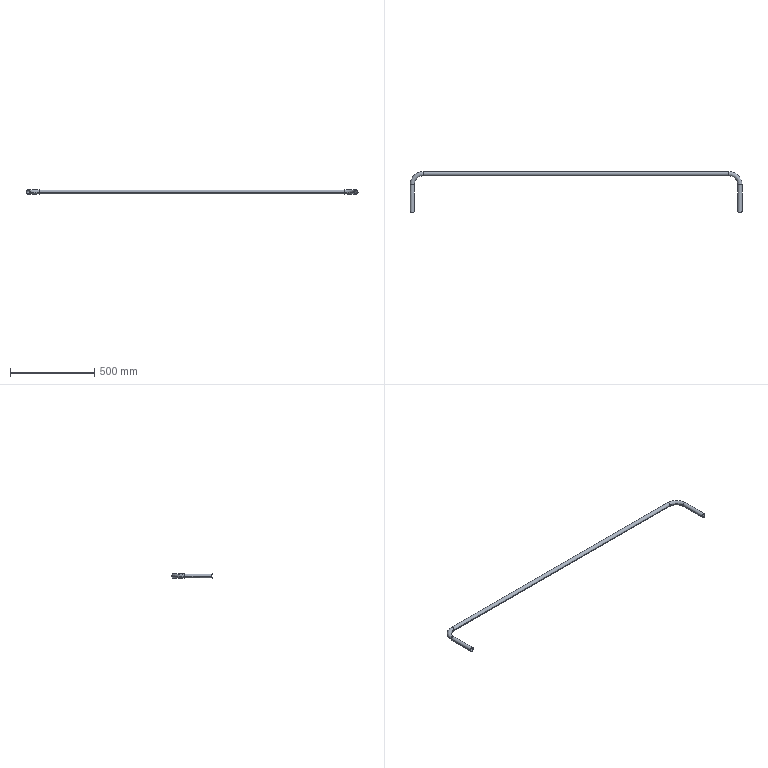Part | NX | features BREP 1 | 1 solid | 22 faces | box 1965 x 241.706 x 25.4 mm | volume 263109 mm3 | cylinder 14 | torus 8 | commonest cylinder face diameters 22.403 x6 25.4 x6 38.1 x2
STEP:
#1=CARTESIAN_POINT('',(-956.945,174.752,0.));
#2=VERTEX_POINT('',#1);
#3=CARTESIAN_POINT('',(-956.945,15.875,0.));
#4=VERTEX_POINT('',#3);
#5=CARTESIAN_POINT('',(-956.945,15.875,0.));
#6=DIRECTION('',(0.,1.,0.));
#7=VECTOR('',#6,1000.);
#8=LINE('',#5,#7);
#9=EDGE_CURVE('',#2,#4,#8,.F.);
#10=ORIENTED_EDGE('',*,*,#9,.F.);
#11=CARTESIAN_POINT('',(-982.345,174.752,0.));
#12=VERTEX_POINT('',#11);
#13=CARTESIAN_POINT('',(-969.645,174.752,0.));
#14=DIRECTION('',(0.,1.,0.));
#15=DIRECTION('',(-1.,0.,0.));
#16=AXIS2_PLACEMENT_3D('',#13,#14,#15);
#17=CIRCLE('',#16,12.7);
#18=EDGE_CURVE('',#12,#2,#17,.T.);
#19=ORIENTED_EDGE('',*,*,#18,.F.);
#20=CARTESIAN_POINT('',(-982.345,15.875,0.));
#21=VERTEX_POINT('',#20);
#22=CARTESIAN_POINT('',(-982.345,15.875,0.));
#23=DIRECTION('',(0.,1.,0.));
#24=VECTOR('',#23,1000.);
#25=LINE('',#22,#24);
#26=EDGE_CURVE('',#12,#21,#25,.F.);
#27=ORIENTED_EDGE('',*,*,#26,.T.);
#28=CARTESIAN_POINT('',(-982.345,15.875,0.));
#29=CARTESIAN_POINT('',(-982.345,15.875,0.8172));
#30=CARTESIAN_POINT('',(-982.197,15.772,2.464));
#31=CARTESIAN_POINT('',(-981.526,15.337,4.623));
#32=CARTESIAN_POINT('',(-980.908,14.947,5.892));
#33=CARTESIAN_POINT('',(-980.483,14.687,6.633));
#34=CARTESIAN_POINT('',(-980.08,14.445,7.248));
#35=CARTESIAN_POINT('',(-979.807,14.285,7.623));
#36=CARTESIAN_POINT('',(-979.423,14.062,8.115));
#37=CARTESIAN_POINT('',(-978.957,13.802,8.644));
#38=CARTESIAN_POINT('',(-978.566,13.59,9.049));
#39=CARTESIAN_POINT('',(-978.055,13.326,9.521));
#40=CARTESIAN_POINT('',(-977.617,13.108,9.893));
#41=CARTESIAN_POINT('',(-977.12,12.872,10.274));
#42=CARTESIAN_POINT('',(-976.753,12.704,10.527));
#43=CARTESIAN_POINT('',(-976.498,12.592,10.692));
#44=CARTESIAN_POINT('',(-976.434,12.564,10.734));
#45=CARTESIAN_POINT('',(-976.069,12.41,10.958));
#46=CARTESIAN_POINT('',(-975.694,12.26,11.17));
#47=CARTESIAN_POINT('',(-974.997,11.995,11.531));
#48=CARTESIAN_POINT('',(-974.162,11.714,11.889));
#49=CARTESIAN_POINT('',(-972.932,11.385,12.29));
#50=CARTESIAN_POINT('',(-971.375,11.099,12.624));
#51=CARTESIAN_POINT('',(-969.463,10.963,12.763));
#52=CARTESIAN_POINT('',(-967.657,11.135,12.582));
#53=CARTESIAN_POINT('',(-966.133,11.438,12.227));
#54=CARTESIAN_POINT('',(-964.915,11.78,11.805));
#55=CARTESIAN_POINT('',(-964.127,12.055,11.451));
#56=CARTESIAN_POINT('',(-963.454,12.315,11.092));
#57=CARTESIAN_POINT('',(-963.097,12.461,10.884));
#58=CARTESIAN_POINT('',(-962.737,12.615,10.658));
#59=CARTESIAN_POINT('',(-962.705,12.63,10.636));
#60=CARTESIAN_POINT('',(-962.476,12.732,10.485));
#61=CARTESIAN_POINT('',(-962.132,12.89,10.246));
#62=CARTESIAN_POINT('',(-961.638,13.126,9.864));
#63=CARTESIAN_POINT('',(-961.2,13.344,9.491));
#64=CARTESIAN_POINT('',(-960.795,13.554,9.112));
#65=CARTESIAN_POINT('',(-960.557,13.682,8.874));
#66=CARTESIAN_POINT('',(-960.215,13.867,8.513));
#67=CARTESIAN_POINT('',(-959.856,14.069,8.099));
#68=CARTESIAN_POINT('',(-959.472,14.291,7.608));
#69=CARTESIAN_POINT('',(-959.201,14.451,7.233));
#70=CARTESIAN_POINT('',(-958.801,14.69,6.624));
#71=CARTESIAN_POINT('',(-958.379,14.949,5.885));
#72=CARTESIAN_POINT('',(-957.946,15.222,4.997));
#73=CARTESIAN_POINT('',(-957.48,15.521,3.727));
#74=CARTESIAN_POINT('',(-957.066,15.791,2.074));
#75=CARTESIAN_POINT('',(-956.945,15.875,0.8178));
#76=CARTESIAN_POINT('',(-956.945,15.875,0.));
#77=B_SPLINE_CURVE_WITH_KNOTS('',3,(#28,#29,#30,#31,#32,#33,#34,#35,#36,#37,#38,#39,#40,#41,#42,#43,#44,#45,#46,#47,#48,#49,#50,#51,#52,#53,#54,#55,#56,#57,#58,#59,#60,#61,#62,#63,#64,#65,#66,#67,#68,#69,#70,#71,#72,#73,#74,#75,#76),.UNSPECIFIED.,.F.,.F.,(4,1,1,1,1,1,1,1,1,1,1,1,1,1,1,1,1,1,1,1,1,1,1,1,1,1,1,1,1,1,1,1,1,1,1,1,1,1,1,1,1,1,1,1,1,1,4),(0.,0.0625,0.125,0.1562,0.1719,0.1875,0.2031,0.2188,0.2344,0.25,0.2578,0.2656,0.2812,0.2969,0.3047,0.3125,0.3203,0.3281,0.3438,0.375,0.4062,0.4375,0.5,0.5625,0.5938,0.625,0.6562,0.6719,0.6797,0.6875,0.6953,0.7031,0.7188,0.7344,0.7422,0.75,0.7578,0.7656,0.7812,0.7969,0.8125,0.8281,0.8438,0.875,0.9062,0.9375,1.),.UNSPECIFIED.);
#78=EDGE_CURVE('',#21,#4,#77,.T.);
#79=ORIENTED_EDGE('',*,*,#78,.T.);
#80=EDGE_LOOP('',(#10,#19,#27,#79));
#81=FACE_BOUND('',#80,.T.);
#82=CARTESIAN_POINT('',(-969.645,0.,0.));
#83=DIRECTION('',(0.,1.,0.));
#84=DIRECTION('',(-1.,0.,0.));
#85=AXIS2_PLACEMENT_3D('',#82,#83,#84);
#86=CYLINDRICAL_SURFACE('',#85,12.7);
#87=ADVANCED_FACE('',(#81),#86,.T.);
#88=CARTESIAN_POINT('',(-982.345,15.875,0.));
#89=CARTESIAN_POINT('',(-982.345,15.875,-1.695));
#90=CARTESIAN_POINT('',(-981.677,15.422,-5.04));
#91=CARTESIAN_POINT('',(-978.692,13.557,-9.433));
#92=CARTESIAN_POINT('',(-974.201,11.514,-12.195));
#93=CARTESIAN_POINT('',(-969.57,10.77,-12.963));
#94=CARTESIAN_POINT('',(-964.988,11.553,-12.151));
#95=CARTESIAN_POINT('',(-960.544,13.589,-9.376));
#96=CARTESIAN_POINT('',(-957.6,15.431,-4.995));
#97=CARTESIAN_POINT('',(-956.945,15.875,-1.68));
#98=CARTESIAN_POINT('',(-956.945,15.875,0.));
#99=B_SPLINE_CURVE_WITH_KNOTS('',3,(#88,#89,#90,#91,#92,#93,#94,#95,#96,#97,#98),.UNSPECIFIED.,.F.,.F.,(4,1,1,1,1,1,1,1,4),(0.,0.125,0.25,0.375,0.5,0.625,0.75,0.875,1.),.UNSPECIFIED.);
#100=EDGE_CURVE('',#4,#21,#99,.F.);
#101=ORIENTED_EDGE('',*,*,#100,.F.);
#102=ORIENTED_EDGE('',*,*,#78,.F.);
#103=EDGE_LOOP('',(#101,#102));
#104=FACE_BOUND('',#103,.T.);
#105=CARTESIAN_POINT('',(-958.444,15.875,0.));
#106=VERTEX_POINT('',#105);
#107=CARTESIAN_POINT('',(-980.846,15.875,0.));
#108=VERTEX_POINT('',#107);
#109=CARTESIAN_POINT('',(-980.846,15.875,0.));
#110=CARTESIAN_POINT('',(-980.846,15.875,1.513));
#111=CARTESIAN_POINT('',(-980.232,15.505,4.51));
#112=CARTESIAN_POINT('',(-977.61,14.087,8.313));
#113=CARTESIAN_POINT('',(-973.75,12.609,10.717));
#114=CARTESIAN_POINT('',(-969.642,12.045,11.446));
#115=CARTESIAN_POINT('',(-965.514,12.615,10.707));
#116=CARTESIAN_POINT('',(-961.681,14.087,8.312));
#117=CARTESIAN_POINT('',(-959.051,15.509,4.496));
#118=CARTESIAN_POINT('',(-958.444,15.875,1.51));
#119=CARTESIAN_POINT('',(-958.444,15.875,0.));
#120=B_SPLINE_CURVE_WITH_KNOTS('',3,(#109,#110,#111,#112,#113,#114,#115,#116,#117,#118,#119),.UNSPECIFIED.,.F.,.F.,(4,1,1,1,1,1,1,1,4),(0.,0.125,0.25,0.375,0.5,0.625,0.75,0.875,1.),.UNSPECIFIED.);
#121=EDGE_CURVE('',#106,#108,#120,.F.);
#122=ORIENTED_EDGE('',*,*,#121,.F.);
#123=CARTESIAN_POINT('',(-958.444,15.875,0.));
#124=CARTESIAN_POINT('',(-958.444,15.875,-1.476));
#125=CARTESIAN_POINT('',(-959.015,15.532,-4.378));
#126=CARTESIAN_POINT('',(-961.576,14.135,-8.222));
#127=CARTESIAN_POINT('',(-965.462,12.632,-10.686));
#128=CARTESIAN_POINT('',(-969.537,12.04,-11.451));
#129=CARTESIAN_POINT('',(-973.803,12.611,-10.719));
#130=CARTESIAN_POINT('',(-977.735,14.147,-8.202));
#131=CARTESIAN_POINT('',(-980.277,15.533,-4.367));
#132=CARTESIAN_POINT('',(-980.846,15.875,-1.472));
#133=CARTESIAN_POINT('',(-980.846,15.875,0.));
#134=B_SPLINE_CURVE_WITH_KNOTS('',3,(#123,#124,#125,#126,#127,#128,#129,#130,#131,#132,#133),.UNSPECIFIED.,.F.,.F.,(4,1,1,1,1,1,1,1,4),(0.,0.125,0.25,0.375,0.5,0.625,0.75,0.875,1.),.UNSPECIFIED.);
#135=EDGE_CURVE('',#108,#106,#134,.F.);
#136=ORIENTED_EDGE('',*,*,#135,.F.);
#137=EDGE_LOOP('',(#122,#136));
#138=FACE_BOUND('',#137,.T.);
#139=CARTESIAN_POINT('',(1178.814,-3.175,0.));
#140=DIRECTION('',(1.,0.,0.));
#141=DIRECTION('',(0.,0.,-1.));
#142=AXIS2_PLACEMENT_3D('',#139,#140,#141);
#143=CYLINDRICAL_SURFACE('',#142,19.05);
#144=ADVANCED_FACE('',(#104,#138),#143,.F.);
#145=CARTESIAN_POINT('',(982.345,15.875,0.));
#146=VERTEX_POINT('',#145);
#147=CARTESIAN_POINT('',(956.945,15.875,0.));
#148=VERTEX_POINT('',#147);
#149=CARTESIAN_POINT('',(956.945,15.875,0.));
#150=CARTESIAN_POINT('',(956.945,15.875,-1.694));
#151=CARTESIAN_POINT('',(957.616,15.42,-5.043));
#152=CARTESIAN_POINT('',(960.585,13.565,-9.414));
#153=CARTESIAN_POINT('',(965.036,11.537,-12.168));
#154=CARTESIAN_POINT('',(969.617,10.769,-12.963));
#155=CARTESIAN_POINT('',(974.249,11.53,-12.178));
#156=CARTESIAN_POINT('',(978.733,13.581,-9.394));
#157=CARTESIAN_POINT('',(981.691,15.432,-4.995));
#158=CARTESIAN_POINT('',(982.345,15.875,-1.682));
#159=CARTESIAN_POINT('',(982.345,15.875,0.));
#160=B_SPLINE_CURVE_WITH_KNOTS('',3,(#149,#150,#151,#152,#153,#154,#155,#156,#157,#158,#159),.UNSPECIFIED.,.F.,.F.,(4,1,1,1,1,1,1,1,4),(0.,0.125,0.25,0.375,0.5,0.625,0.75,0.875,1.),.UNSPECIFIED.);
#161=EDGE_CURVE('',#146,#148,#160,.F.);
#162=ORIENTED_EDGE('',*,*,#161,.F.);
#163=CARTESIAN_POINT('',(982.345,15.875,0.));
#164=CARTESIAN_POINT('',(982.345,15.875,1.704));
#165=CARTESIAN_POINT('',(981.657,15.408,5.088));
#166=CARTESIAN_POINT('',(978.7,13.566,9.4));
#167=CARTESIAN_POINT('',(974.367,11.587,12.109));
#168=CARTESIAN_POINT('',(969.865,10.768,12.966));
#169=CARTESIAN_POINT('',(965.12,11.494,12.222));
#170=CARTESIAN_POINT('',(960.591,13.562,9.425));
#171=CARTESIAN_POINT('',(957.623,15.415,5.06));
#172=CARTESIAN_POINT('',(956.945,15.875,1.699));
#173=CARTESIAN_POINT('',(956.945,15.875,0.));
#174=B_SPLINE_CURVE_WITH_KNOTS('',3,(#163,#164,#165,#166,#167,#168,#169,#170,#171,#172,#173),.UNSPECIFIED.,.F.,.F.,(4,1,1,1,1,1,1,1,4),(0.,0.125,0.25,0.375,0.5,0.625,0.75,0.875,1.),.UNSPECIFIED.);
#175=EDGE_CURVE('',#148,#146,#174,.F.);
#176=ORIENTED_EDGE('',*,*,#175,.F.);
#177=EDGE_LOOP('',(#162,#176));
#178=FACE_BOUND('',#177,.T.);
#179=CARTESIAN_POINT('',(980.846,15.875,0.));
#180=VERTEX_POINT('',#179);
#181=CARTESIAN_POINT('',(958.444,15.875,0.));
#182=VERTEX_POINT('',#181);
#183=CARTESIAN_POINT('',(958.444,15.875,0.));
#184=CARTESIAN_POINT('',(958.444,15.875,1.51));
#185=CARTESIAN_POINT('',(959.051,15.509,4.496));
#186=CARTESIAN_POINT('',(961.681,14.087,8.312));
#187=CARTESIAN_POINT('',(965.514,12.615,10.707));
#188=CARTESIAN_POINT('',(969.642,12.045,11.446));
#189=CARTESIAN_POINT('',(973.75,12.609,10.717));
#190=CARTESIAN_POINT('',(977.61,14.087,8.313));
#191=CARTESIAN_POINT('',(980.232,15.505,4.51));
#192=CARTESIAN_POINT('',(980.846,15.875,1.514));
#193=CARTESIAN_POINT('',(980.846,15.875,0.));
#194=B_SPLINE_CURVE_WITH_KNOTS('',3,(#183,#184,#185,#186,#187,#188,#189,#190,#191,#192,#193),.UNSPECIFIED.,.F.,.F.,(4,1,1,1,1,1,1,1,4),(0.,0.125,0.25,0.375,0.5,0.625,0.75,0.875,1.),.UNSPECIFIED.);
#195=EDGE_CURVE('',#180,#182,#194,.F.);
#196=ORIENTED_EDGE('',*,*,#195,.F.);
#197=CARTESIAN_POINT('',(980.846,15.875,0.));
#198=CARTESIAN_POINT('',(980.846,15.875,-1.475));
#199=CARTESIAN_POINT('',(980.274,15.532,-4.378));
#200=CARTESIAN_POINT('',(977.72,14.139,-8.214));
#201=CARTESIAN_POINT('',(973.844,12.635,-10.682));
#202=CARTESIAN_POINT('',(969.746,12.04,-11.45));
#203=CARTESIAN_POINT('',(965.517,12.604,-10.728));
#204=CARTESIAN_POINT('',(961.566,14.14,-8.217));
#205=CARTESIAN_POINT('',(959.016,15.531,-4.376));
#206=CARTESIAN_POINT('',(958.444,15.875,-1.476));
#207=CARTESIAN_POINT('',(958.444,15.875,0.));
#208=B_SPLINE_CURVE_WITH_KNOTS('',3,(#197,#198,#199,#200,#201,#202,#203,#204,#205,#206,#207),.UNSPECIFIED.,.F.,.F.,(4,1,1,1,1,1,1,1,4),(0.,0.125,0.25,0.375,0.5,0.625,0.75,0.875,1.),.UNSPECIFIED.);
#209=EDGE_CURVE('',#182,#180,#208,.F.);
#210=ORIENTED_EDGE('',*,*,#209,.F.);
#211=EDGE_LOOP('',(#196,#210));
#212=FACE_BOUND('',#211,.T.);
#213=CARTESIAN_POINT('',(1178.814,-3.175,0.));
#214=DIRECTION('',(1.,0.,0.));
#215=DIRECTION('',(0.,0.,-1.));
#216=AXIS2_PLACEMENT_3D('',#213,#214,#215);
#217=CYLINDRICAL_SURFACE('',#216,19.05);
#218=ADVANCED_FACE('',(#178,#212),#217,.F.);
#219=ORIENTED_EDGE('',*,*,#26,.F.);
#220=CARTESIAN_POINT('',(-969.645,174.752,0.));
#221=DIRECTION('',(0.,1.,0.));
#222=DIRECTION('',(1.,0.,0.));
#223=AXIS2_PLACEMENT_3D('',#220,#221,#222);
#224=CIRCLE('',#223,12.7);
#225=EDGE_CURVE('',#2,#12,#224,.T.);
#226=ORIENTED_EDGE('',*,*,#225,.F.);
#227=ORIENTED_EDGE('',*,*,#9,.T.);
#228=ORIENTED_EDGE('',*,*,#100,.T.);
#229=EDGE_LOOP('',(#219,#226,#227,#228));
#230=FACE_BOUND('',#229,.T.);
#231=CARTESIAN_POINT('',(-969.645,0.,0.));
#232=DIRECTION('',(0.,1.,0.));
#233=DIRECTION('',(-1.,0.,0.));
#234=AXIS2_PLACEMENT_3D('',#231,#232,#233);
#235=CYLINDRICAL_SURFACE('',#234,12.7);
#236=ADVANCED_FACE('',(#230),#235,.T.);
#237=CARTESIAN_POINT('',(-904.367,252.73,0.));
#238=VERTEX_POINT('',#237);
#239=CARTESIAN_POINT('',(-904.367,174.752,0.));
#240=DIRECTION('',(0.,0.,-1.));
#241=DIRECTION('',(-1.,0.,0.));
#242=AXIS2_PLACEMENT_3D('',#239,#240,#241);
#243=CIRCLE('',#242,77.978);
#244=EDGE_CURVE('',#12,#238,#243,.T.);
#245=ORIENTED_EDGE('',*,*,#244,.T.);
#246=CARTESIAN_POINT('',(-904.367,227.33,0.));
#247=VERTEX_POINT('',#246);
#248=CARTESIAN_POINT('',(-904.367,240.03,0.));
#249=DIRECTION('',(1.,0.,0.));
#250=DIRECTION('',(0.,-1.,0.));
#251=AXIS2_PLACEMENT_3D('',#248,#249,#250);
#252=CIRCLE('',#251,12.7);
#253=EDGE_CURVE('',#247,#238,#252,.T.);
#254=ORIENTED_EDGE('',*,*,#253,.F.);
#255=CARTESIAN_POINT('',(-904.367,174.752,0.));
#256=DIRECTION('',(0.,0.,-1.));
#257=DIRECTION('',(-1.,0.,0.));
#258=AXIS2_PLACEMENT_3D('',#255,#256,#257);
#259=CIRCLE('',#258,52.578);
#260=EDGE_CURVE('',#2,#247,#259,.T.);
#261=ORIENTED_EDGE('',*,*,#260,.F.);
#262=ORIENTED_EDGE('',*,*,#225,.T.);
#263=EDGE_LOOP('',(#245,#254,#261,#262));
#264=FACE_BOUND('',#263,.T.);
#265=CARTESIAN_POINT('',(-904.367,174.752,0.));
#266=DIRECTION('',(0.,0.,-1.));
#267=DIRECTION('',(1.,0.,0.));
#268=AXIS2_PLACEMENT_3D('',#265,#266,#267);
#269=TOROIDAL_SURFACE('',#268,65.278,12.7);
#270=ADVANCED_FACE('',(#264),#269,.T.);
#271=ORIENTED_EDGE('',*,*,#260,.T.);
#272=CARTESIAN_POINT('',(-904.367,240.03,0.));
#273=DIRECTION('',(1.,0.,0.));
#274=DIRECTION('',(0.,1.,0.));
#275=AXIS2_PLACEMENT_3D('',#272,#273,#274);
#276=CIRCLE('',#275,12.7);
#277=EDGE_CURVE('',#238,#247,#276,.T.);
#278=ORIENTED_EDGE('',*,*,#277,.F.);
#279=ORIENTED_EDGE('',*,*,#244,.F.);
#280=ORIENTED_EDGE('',*,*,#18,.T.);
#281=EDGE_LOOP('',(#271,#278,#279,#280));
#282=FACE_BOUND('',#281,.T.);
#283=CARTESIAN_POINT('',(-904.367,174.752,0.));
#284=DIRECTION('',(0.,0.,-1.));
#285=DIRECTION('',(1.,0.,0.));
#286=AXIS2_PLACEMENT_3D('',#283,#284,#285);
#287=TOROIDAL_SURFACE('',#286,65.278,12.7);
#288=ADVANCED_FACE('',(#282),#287,.T.);
#289=CARTESIAN_POINT('',(904.367,227.33,0.));
#290=VERTEX_POINT('',#289);
#291=CARTESIAN_POINT('',(-904.367,227.33,0.));
#292=DIRECTION('',(1.,0.,0.));
#293=VECTOR('',#292,1000.);
#294=LINE('',#291,#293);
#295=EDGE_CURVE('',#247,#290,#294,.T.);
#296=ORIENTED_EDGE('',*,*,#295,.T.);
#297=CARTESIAN_POINT('',(904.367,252.73,0.));
#298=VERTEX_POINT('',#297);
#299=CARTESIAN_POINT('',(904.367,240.03,0.));
#300=DIRECTION('',(1.,0.,0.));
#301=DIRECTION('',(0.,1.,0.));
#302=AXIS2_PLACEMENT_3D('',#299,#300,#301);
#303=CIRCLE('',#302,12.7);
#304=EDGE_CURVE('',#298,#290,#303,.T.);
#305=ORIENTED_EDGE('',*,*,#304,.F.);
#306=CARTESIAN_POINT('',(-904.367,252.73,0.));
#307=DIRECTION('',(1.,0.,0.));
#308=VECTOR('',#307,1000.);
#309=LINE('',#306,#308);
#310=EDGE_CURVE('',#238,#298,#309,.T.);
#311=ORIENTED_EDGE('',*,*,#310,.F.);
#312=ORIENTED_EDGE('',*,*,#277,.T.);
#313=EDGE_LOOP('',(#296,#305,#311,#312));
#314=FACE_BOUND('',#313,.T.);
#315=CARTESIAN_POINT('',(-904.367,240.03,0.));
#316=DIRECTION('',(1.,0.,0.));
#317=DIRECTION('',(0.,1.,0.));
#318=AXIS2_PLACEMENT_3D('',#315,#316,#317);
#319=CYLINDRICAL_SURFACE('',#318,12.7);
#320=ADVANCED_FACE('',(#314),#319,.T.);
#321=ORIENTED_EDGE('',*,*,#310,.T.);
#322=CARTESIAN_POINT('',(904.367,240.03,0.));
#323=DIRECTION('',(1.,0.,0.));
#324=DIRECTION('',(0.,-1.,0.));
#325=AXIS2_PLACEMENT_3D('',#322,#323,#324);
#326=CIRCLE('',#325,12.7);
#327=EDGE_CURVE('',#290,#298,#326,.T.);
#328=ORIENTED_EDGE('',*,*,#327,.F.);
#329=ORIENTED_EDGE('',*,*,#295,.F.);
#330=ORIENTED_EDGE('',*,*,#253,.T.);
#331=EDGE_LOOP('',(#321,#328,#329,#330));
#332=FACE_BOUND('',#331,.T.);
#333=CARTESIAN_POINT('',(-904.367,240.03,0.));
#334=DIRECTION('',(1.,0.,0.));
#335=DIRECTION('',(0.,1.,0.));
#336=AXIS2_PLACEMENT_3D('',#333,#334,#335);
#337=CYLINDRICAL_SURFACE('',#336,12.7);
#338=ADVANCED_FACE('',(#332),#337,.T.);
#339=CARTESIAN_POINT('',(982.345,174.752,0.));
#340=VERTEX_POINT('',#339);
#341=CARTESIAN_POINT('',(904.367,174.752,0.));
#342=DIRECTION('',(0.,0.,-1.));
#343=DIRECTION('',(0.,1.,0.));
#344=AXIS2_PLACEMENT_3D('',#341,#342,#343);
#345=CIRCLE('',#344,77.978);
#346=EDGE_CURVE('',#340,#298,#345,.F.);
#347=ORIENTED_EDGE('',*,*,#346,.F.);
#348=CARTESIAN_POINT('',(956.945,174.752,0.));
#349=VERTEX_POINT('',#348);
#350=CARTESIAN_POINT('',(969.645,174.752,0.));
#351=DIRECTION('',(0.,-1.,0.));
#352=DIRECTION('',(-1.,0.,0.));
#353=AXIS2_PLACEMENT_3D('',#350,#351,#352);
#354=CIRCLE('',#353,12.7);
#355=EDGE_CURVE('',#349,#340,#354,.T.);
#356=ORIENTED_EDGE('',*,*,#355,.F.);
#357=CARTESIAN_POINT('',(904.367,174.752,0.));
#358=DIRECTION('',(0.,0.,-1.));
#359=DIRECTION('',(0.,1.,0.));
#360=AXIS2_PLACEMENT_3D('',#357,#358,#359);
#361=CIRCLE('',#360,52.578);
#362=EDGE_CURVE('',#349,#290,#361,.F.);
#363=ORIENTED_EDGE('',*,*,#362,.T.);
#364=ORIENTED_EDGE('',*,*,#327,.T.);
#365=EDGE_LOOP('',(#347,#356,#363,#364));
#366=FACE_BOUND('',#365,.T.);
#367=CARTESIAN_POINT('',(904.367,174.752,0.));
#368=DIRECTION('',(0.,0.,-1.));
#369=DIRECTION('',(0.,-1.,0.));
#370=AXIS2_PLACEMENT_3D('',#367,#368,#369);
#371=TOROIDAL_SURFACE('',#370,65.278,12.7);
#372=ADVANCED_FACE('',(#366),#371,.T.);
#373=ORIENTED_EDGE('',*,*,#362,.F.);
#374=CARTESIAN_POINT('',(969.645,174.752,0.));
#375=DIRECTION('',(0.,-1.,0.));
#376=DIRECTION('',(1.,0.,0.));
#377=AXIS2_PLACEMENT_3D('',#374,#375,#376);
#378=CIRCLE('',#377,12.7);
#379=EDGE_CURVE('',#340,#349,#378,.T.);
#380=ORIENTED_EDGE('',*,*,#379,.F.);
#381=ORIENTED_EDGE('',*,*,#346,.T.);
#382=ORIENTED_EDGE('',*,*,#304,.T.);
#383=EDGE_LOOP('',(#373,#380,#381,#382));
#384=FACE_BOUND('',#383,.T.);
#385=CARTESIAN_POINT('',(904.367,174.752,0.));
#386=DIRECTION('',(0.,0.,-1.));
#387=DIRECTION('',(0.,-1.,0.));
#388=AXIS2_PLACEMENT_3D('',#385,#386,#387);
#389=TOROIDAL_SURFACE('',#388,65.278,12.7);
#390=ADVANCED_FACE('',(#384),#389,.T.);
#391=CARTESIAN_POINT('',(982.345,174.752,0.));
#392=DIRECTION('',(0.,-1.,0.));
#393=VECTOR('',#392,1000.);
#394=LINE('',#391,#393);
#395=EDGE_CURVE('',#146,#340,#394,.F.);
#396=ORIENTED_EDGE('',*,*,#395,.T.);
#397=ORIENTED_EDGE('',*,*,#379,.T.);
#398=CARTESIAN_POINT('',(956.945,174.752,0.));
#399=DIRECTION('',(0.,-1.,0.));
#400=VECTOR('',#399,1000.);
#401=LINE('',#398,#400);
#402=EDGE_CURVE('',#148,#349,#401,.F.);
#403=ORIENTED_EDGE('',*,*,#402,.F.);
#404=ORIENTED_EDGE('',*,*,#175,.T.);
#405=EDGE_LOOP('',(#396,#397,#403,#404));
#406=FACE_BOUND('',#405,.T.);
#407=CARTESIAN_POINT('',(969.645,174.752,0.));
#408=DIRECTION('',(0.,-1.,0.));
#409=DIRECTION('',(1.,0.,0.));
#410=AXIS2_PLACEMENT_3D('',#407,#408,#409);
#411=CYLINDRICAL_SURFACE('',#410,12.7);
#412=ADVANCED_FACE('',(#406),#411,.T.);
#413=ORIENTED_EDGE('',*,*,#402,.T.);
#414=ORIENTED_EDGE('',*,*,#355,.T.);
#415=ORIENTED_EDGE('',*,*,#395,.F.);
#416=ORIENTED_EDGE('',*,*,#161,.T.);
#417=EDGE_LOOP('',(#413,#414,#415,#416));
#418=FACE_BOUND('',#417,.T.);
#419=CARTESIAN_POINT('',(969.645,174.752,0.));
#420=DIRECTION('',(0.,-1.,0.));
#421=DIRECTION('',(1.,0.,0.));
#422=AXIS2_PLACEMENT_3D('',#419,#420,#421);
#423=CYLINDRICAL_SURFACE('',#422,12.7);
#424=ADVANCED_FACE('',(#418),#423,.T.);
#425=CARTESIAN_POINT('',(-958.444,174.752,0.));
#426=VERTEX_POINT('',#425);
#427=CARTESIAN_POINT('',(-958.444,15.875,0.));
#428=DIRECTION('',(0.,1.,0.));
#429=VECTOR('',#428,1000.);
#430=LINE('',#427,#429);
#431=EDGE_CURVE('',#426,#106,#430,.F.);
#432=ORIENTED_EDGE('',*,*,#431,.F.);
#433=CARTESIAN_POINT('',(-980.846,174.752,0.));
#434=VERTEX_POINT('',#433);
#435=CARTESIAN_POINT('',(-969.645,174.752,0.));
#436=DIRECTION('',(0.,-1.,0.));
#437=DIRECTION('',(-1.,0.,0.));
#438=AXIS2_PLACEMENT_3D('',#435,#436,#437);
#439=CIRCLE('',#438,11.201);
#440=EDGE_CURVE('',#434,#426,#439,.T.);
#441=ORIENTED_EDGE('',*,*,#440,.F.);
#442=CARTESIAN_POINT('',(-980.846,15.875,0.));
#443=DIRECTION('',(0.,1.,0.));
#444=VECTOR('',#443,1000.);
#445=LINE('',#442,#444);
#446=EDGE_CURVE('',#434,#108,#445,.F.);
#447=ORIENTED_EDGE('',*,*,#446,.T.);
#448=ORIENTED_EDGE('',*,*,#135,.T.);
#449=EDGE_LOOP('',(#432,#441,#447,#448));
#450=FACE_BOUND('',#449,.T.);
#451=CARTESIAN_POINT('',(-969.645,0.,0.));
#452=DIRECTION('',(0.,1.,0.));
#453=DIRECTION('',(-1.,0.,0.));
#454=AXIS2_PLACEMENT_3D('',#451,#452,#453);
#455=CYLINDRICAL_SURFACE('',#454,11.201);
#456=ADVANCED_FACE('',(#450),#455,.F.);
#457=ORIENTED_EDGE('',*,*,#446,.F.);
#458=CARTESIAN_POINT('',(-969.645,174.752,0.));
#459=DIRECTION('',(0.,-1.,0.));
#460=DIRECTION('',(1.,0.,0.));
#461=AXIS2_PLACEMENT_3D('',#458,#459,#460);
#462=CIRCLE('',#461,11.201);
#463=EDGE_CURVE('',#426,#434,#462,.T.);
#464=ORIENTED_EDGE('',*,*,#463,.F.);
#465=ORIENTED_EDGE('',*,*,#431,.T.);
#466=ORIENTED_EDGE('',*,*,#121,.T.);
#467=EDGE_LOOP('',(#457,#464,#465,#466));
#468=FACE_BOUND('',#467,.T.);
#469=CARTESIAN_POINT('',(-969.645,0.,0.));
#470=DIRECTION('',(0.,1.,0.));
#471=DIRECTION('',(-1.,0.,0.));
#472=AXIS2_PLACEMENT_3D('',#469,#470,#471);
#473=CYLINDRICAL_SURFACE('',#472,11.201);
#474=ADVANCED_FACE('',(#468),#473,.F.);
#475=CARTESIAN_POINT('',(-904.367,251.231,0.));
#476=VERTEX_POINT('',#475);
#477=CARTESIAN_POINT('',(-904.367,174.752,0.));
#478=DIRECTION('',(0.,0.,-1.));
#479=DIRECTION('',(-1.,0.,0.));
#480=AXIS2_PLACEMENT_3D('',#477,#478,#479);
#481=CIRCLE('',#480,76.479);
#482=EDGE_CURVE('',#434,#476,#481,.T.);
#483=ORIENTED_EDGE('',*,*,#482,.T.);
#484=CARTESIAN_POINT('',(-904.367,228.829,0.));
#485=VERTEX_POINT('',#484);
#486=CARTESIAN_POINT('',(-904.367,240.03,0.));
#487=DIRECTION('',(-1.,0.,0.));
#488=DIRECTION('',(0.,-1.,0.));
#489=AXIS2_PLACEMENT_3D('',#486,#487,#488);
#490=CIRCLE('',#489,11.201);
#491=EDGE_CURVE('',#485,#476,#490,.T.);
#492=ORIENTED_EDGE('',*,*,#491,.F.);
#493=CARTESIAN_POINT('',(-904.367,174.752,0.));
#494=DIRECTION('',(0.,0.,-1.));
#495=DIRECTION('',(-1.,0.,0.));
#496=AXIS2_PLACEMENT_3D('',#493,#494,#495);
#497=CIRCLE('',#496,54.077);
#498=EDGE_CURVE('',#426,#485,#497,.T.);
#499=ORIENTED_EDGE('',*,*,#498,.F.);
#500=ORIENTED_EDGE('',*,*,#463,.T.);
#501=EDGE_LOOP('',(#483,#492,#499,#500));
#502=FACE_BOUND('',#501,.T.);
#503=CARTESIAN_POINT('',(-904.367,174.752,0.));
#504=DIRECTION('',(0.,0.,-1.));
#505=DIRECTION('',(1.,0.,0.));
#506=AXIS2_PLACEMENT_3D('',#503,#504,#505);
#507=TOROIDAL_SURFACE('',#506,65.278,11.201);
#508=ADVANCED_FACE('',(#502),#507,.F.);
#509=ORIENTED_EDGE('',*,*,#498,.T.);
#510=CARTESIAN_POINT('',(-904.367,240.03,0.));
#511=DIRECTION('',(-1.,0.,0.));
#512=DIRECTION('',(0.,1.,0.));
#513=AXIS2_PLACEMENT_3D('',#510,#511,#512);
#514=CIRCLE('',#513,11.201);
#515=EDGE_CURVE('',#476,#485,#514,.T.);
#516=ORIENTED_EDGE('',*,*,#515,.F.);
#517=ORIENTED_EDGE('',*,*,#482,.F.);
#518=ORIENTED_EDGE('',*,*,#440,.T.);
#519=EDGE_LOOP('',(#509,#516,#517,#518));
#520=FACE_BOUND('',#519,.T.);
#521=CARTESIAN_POINT('',(-904.367,174.752,0.));
#522=DIRECTION('',(0.,0.,-1.));
#523=DIRECTION('',(1.,0.,0.));
#524=AXIS2_PLACEMENT_3D('',#521,#522,#523);
#525=TOROIDAL_SURFACE('',#524,65.278,11.201);
#526=ADVANCED_FACE('',(#520),#525,.F.);
#527=CARTESIAN_POINT('',(904.367,228.829,0.));
#528=VERTEX_POINT('',#527);
#529=CARTESIAN_POINT('',(-904.367,228.829,0.));
#530=DIRECTION('',(1.,0.,0.));
#531=VECTOR('',#530,1000.);
#532=LINE('',#529,#531);
#533=EDGE_CURVE('',#485,#528,#532,.T.);
#534=ORIENTED_EDGE('',*,*,#533,.T.);
#535=CARTESIAN_POINT('',(904.367,251.231,0.));
#536=VERTEX_POINT('',#535);
#537=CARTESIAN_POINT('',(904.367,240.03,0.));
#538=DIRECTION('',(-1.,0.,0.));
#539=DIRECTION('',(0.,1.,0.));
#540=AXIS2_PLACEMENT_3D('',#537,#538,#539);
#541=CIRCLE('',#540,11.201);
#542=EDGE_CURVE('',#536,#528,#541,.T.);
#543=ORIENTED_EDGE('',*,*,#542,.F.);
#544=CARTESIAN_POINT('',(-904.367,251.231,0.));
#545=DIRECTION('',(1.,0.,0.));
#546=VECTOR('',#545,1000.);
#547=LINE('',#544,#546);
#548=EDGE_CURVE('',#476,#536,#547,.T.);
#549=ORIENTED_EDGE('',*,*,#548,.F.);
#550=ORIENTED_EDGE('',*,*,#515,.T.);
#551=EDGE_LOOP('',(#534,#543,#549,#550));
#552=FACE_BOUND('',#551,.T.);
#553=CARTESIAN_POINT('',(-904.367,240.03,0.));
#554=DIRECTION('',(1.,0.,0.));
#555=DIRECTION('',(0.,1.,0.));
#556=AXIS2_PLACEMENT_3D('',#553,#554,#555);
#557=CYLINDRICAL_SURFACE('',#556,11.201);
#558=ADVANCED_FACE('',(#552),#557,.F.);
#559=ORIENTED_EDGE('',*,*,#548,.T.);
#560=CARTESIAN_POINT('',(904.367,240.03,0.));
#561=DIRECTION('',(-1.,0.,0.));
#562=DIRECTION('',(0.,-1.,0.));
#563=AXIS2_PLACEMENT_3D('',#560,#561,#562);
#564=CIRCLE('',#563,11.201);
#565=EDGE_CURVE('',#528,#536,#564,.T.);
#566=ORIENTED_EDGE('',*,*,#565,.F.);
#567=ORIENTED_EDGE('',*,*,#533,.F.);
#568=ORIENTED_EDGE('',*,*,#491,.T.);
#569=EDGE_LOOP('',(#559,#566,#567,#568));
#570=FACE_BOUND('',#569,.T.);
#571=CARTESIAN_POINT('',(-904.367,240.03,0.));
#572=DIRECTION('',(1.,0.,0.));
#573=DIRECTION('',(0.,1.,0.));
#574=AXIS2_PLACEMENT_3D('',#571,#572,#573);
#575=CYLINDRICAL_SURFACE('',#574,11.201);
#576=ADVANCED_FACE('',(#570),#575,.F.);
#577=CARTESIAN_POINT('',(980.846,174.752,0.));
#578=VERTEX_POINT('',#577);
#579=CARTESIAN_POINT('',(904.367,174.752,0.));
#580=DIRECTION('',(0.,0.,-1.));
#581=DIRECTION('',(0.,1.,0.));
#582=AXIS2_PLACEMENT_3D('',#579,#580,#581);
#583=CIRCLE('',#582,76.479);
#584=EDGE_CURVE('',#578,#536,#583,.F.);
#585=ORIENTED_EDGE('',*,*,#584,.F.);
#586=CARTESIAN_POINT('',(958.444,174.752,0.));
#587=VERTEX_POINT('',#586);
#588=CARTESIAN_POINT('',(969.645,174.752,0.));
#589=DIRECTION('',(0.,1.,0.));
#590=DIRECTION('',(-1.,0.,0.));
#591=AXIS2_PLACEMENT_3D('',#588,#589,#590);
#592=CIRCLE('',#591,11.201);
#593=EDGE_CURVE('',#587,#578,#592,.T.);
#594=ORIENTED_EDGE('',*,*,#593,.F.);
#595=CARTESIAN_POINT('',(904.367,174.752,0.));
#596=DIRECTION('',(0.,0.,-1.));
#597=DIRECTION('',(0.,1.,0.));
#598=AXIS2_PLACEMENT_3D('',#595,#596,#597);
#599=CIRCLE('',#598,54.077);
#600=EDGE_CURVE('',#587,#528,#599,.F.);
#601=ORIENTED_EDGE('',*,*,#600,.T.);
#602=ORIENTED_EDGE('',*,*,#565,.T.);
#603=EDGE_LOOP('',(#585,#594,#601,#602));
#604=FACE_BOUND('',#603,.T.);
#605=CARTESIAN_POINT('',(904.367,174.752,0.));
#606=DIRECTION('',(0.,0.,-1.));
#607=DIRECTION('',(0.,-1.,0.));
#608=AXIS2_PLACEMENT_3D('',#605,#606,#607);
#609=TOROIDAL_SURFACE('',#608,65.278,11.201);
#610=ADVANCED_FACE('',(#604),#609,.F.);
#611=ORIENTED_EDGE('',*,*,#600,.F.);
#612=CARTESIAN_POINT('',(969.645,174.752,0.));
#613=DIRECTION('',(0.,1.,0.));
#614=DIRECTION('',(1.,0.,0.));
#615=AXIS2_PLACEMENT_3D('',#612,#613,#614);
#616=CIRCLE('',#615,11.201);
#617=EDGE_CURVE('',#578,#587,#616,.T.);
#618=ORIENTED_EDGE('',*,*,#617,.F.);
#619=ORIENTED_EDGE('',*,*,#584,.T.);
#620=ORIENTED_EDGE('',*,*,#542,.T.);
#621=EDGE_LOOP('',(#611,#618,#619,#620));
#622=FACE_BOUND('',#621,.T.);
#623=CARTESIAN_POINT('',(904.367,174.752,0.));
#624=DIRECTION('',(0.,0.,-1.));
#625=DIRECTION('',(0.,-1.,0.));
#626=AXIS2_PLACEMENT_3D('',#623,#624,#625);
#627=TOROIDAL_SURFACE('',#626,65.278,11.201);
#628=ADVANCED_FACE('',(#622),#627,.F.);
#629=CARTESIAN_POINT('',(980.846,174.752,0.));
#630=DIRECTION('',(0.,-1.,0.));
#631=VECTOR('',#630,1000.);
#632=LINE('',#629,#631);
#633=EDGE_CURVE('',#180,#578,#632,.F.);
#634=ORIENTED_EDGE('',*,*,#633,.T.);
#635=ORIENTED_EDGE('',*,*,#617,.T.);
#636=CARTESIAN_POINT('',(958.444,174.752,0.));
#637=DIRECTION('',(0.,-1.,0.));
#638=VECTOR('',#637,1000.);
#639=LINE('',#636,#638);
#640=EDGE_CURVE('',#182,#587,#639,.F.);
#641=ORIENTED_EDGE('',*,*,#640,.F.);
#642=ORIENTED_EDGE('',*,*,#209,.T.);
#643=EDGE_LOOP('',(#634,#635,#641,#642));
#644=FACE_BOUND('',#643,.T.);
#645=CARTESIAN_POINT('',(969.645,174.752,0.));
#646=DIRECTION('',(0.,-1.,0.));
#647=DIRECTION('',(1.,0.,0.));
#648=AXIS2_PLACEMENT_3D('',#645,#646,#647);
#649=CYLINDRICAL_SURFACE('',#648,11.201);
#650=ADVANCED_FACE('',(#644),#649,.F.);
#651=ORIENTED_EDGE('',*,*,#640,.T.);
#652=ORIENTED_EDGE('',*,*,#593,.T.);
#653=ORIENTED_EDGE('',*,*,#633,.F.);
#654=ORIENTED_EDGE('',*,*,#195,.T.);
#655=EDGE_LOOP('',(#651,#652,#653,#654));
#656=FACE_BOUND('',#655,.T.);
#657=CARTESIAN_POINT('',(969.645,174.752,0.));
#658=DIRECTION('',(0.,-1.,0.));
#659=DIRECTION('',(1.,0.,0.));
#660=AXIS2_PLACEMENT_3D('',#657,#658,#659);
#661=CYLINDRICAL_SURFACE('',#660,11.201);
#662=ADVANCED_FACE('',(#656),#661,.F.);
#663=CLOSED_SHELL('',(#87,#144,#218,#236,#270,#288,#320,#338,#372,#390,#412,#424,#456,#474,#508,#526,#558,#576,#610,#628,#650,#662));
#664=MANIFOLD_SOLID_BREP('',#663);
#665=(LENGTH_UNIT()NAMED_UNIT(*)SI_UNIT(.MILLI.,.METRE.));
#666=UNCERTAINTY_MEASURE_WITH_UNIT(LENGTH_MEASURE(0.0508),#665,'','');
#667=(NAMED_UNIT(*)PLANE_ANGLE_UNIT()SI_UNIT($,.RADIAN.));
#668=(NAMED_UNIT(*)SI_UNIT($,.STERADIAN.)SOLID_ANGLE_UNIT());
#669=(GEOMETRIC_REPRESENTATION_CONTEXT(3)GLOBAL_UNCERTAINTY_ASSIGNED_CONTEXT((#666))GLOBAL_UNIT_ASSIGNED_CONTEXT((#665,#667,#668))REPRESENTATION_CONTEXT('',''));
#670=ADVANCED_BREP_SHAPE_REPRESENTATION('',(#664),#669);